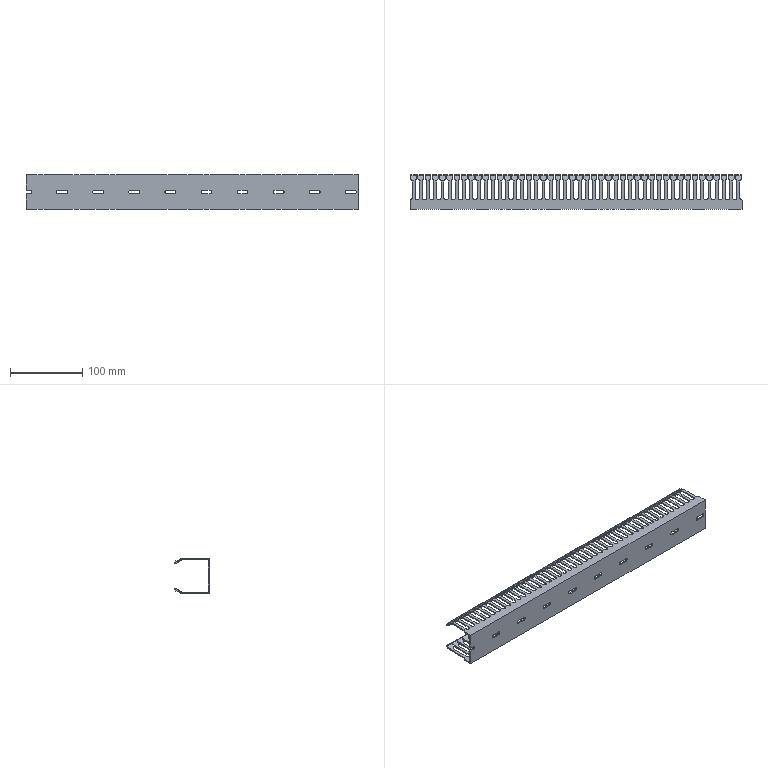Part | STEP file | Cable tray1_1495 | 1 solid | 1384 faces | box 460 x 47.5 x 48 mm | volume 74252 mm3 | plane 949 | cylinder 435 | commonest cylinder face diameters 6 x278 2 x138 5 x19